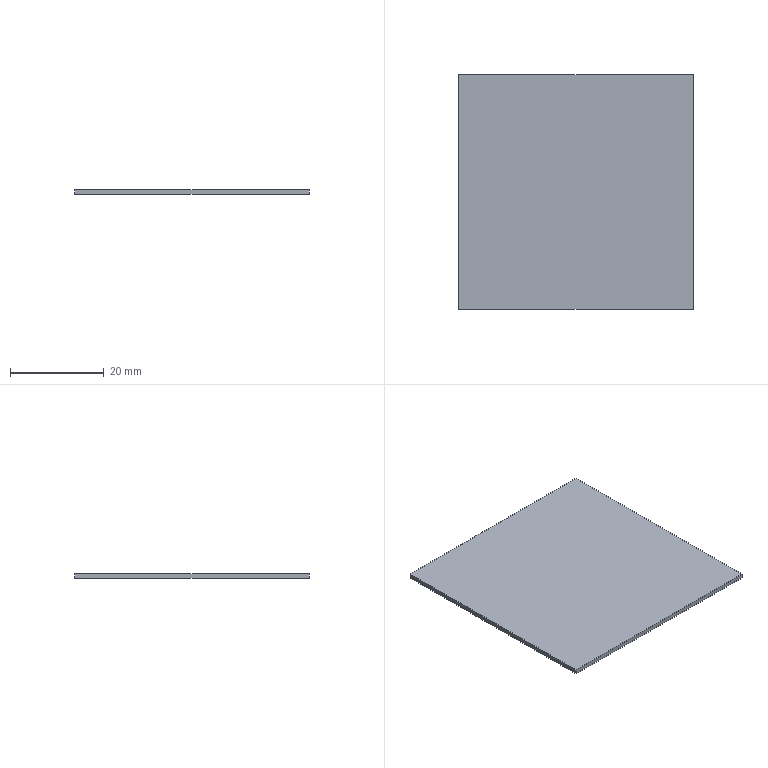Part | SolidWorks | features Extrusion 1 | 1 solid | 6 faces | box 50 x 50 x 1 mm | volume 2500 mm3 | plane 6
STEP:
#1=CARTESIAN_POINT('',(25.,-25.,0.));
#2=VERTEX_POINT('',#1);
#3=CARTESIAN_POINT('',(25.,25.,0.));
#4=VERTEX_POINT('',#3);
#5=CARTESIAN_POINT('',(25.,-25.,0.));
#6=DIRECTION('',(0.,1.,0.));
#7=VECTOR('',#6,1000.);
#8=LINE('',#5,#7);
#9=EDGE_CURVE('',#2,#4,#8,.T.);
#10=ORIENTED_EDGE('',*,*,#9,.T.);
#11=CARTESIAN_POINT('',(25.,25.,1.));
#12=VERTEX_POINT('',#11);
#13=CARTESIAN_POINT('',(25.,25.,1.));
#14=DIRECTION('',(0.,0.,-1.));
#15=VECTOR('',#14,1000.);
#16=LINE('',#13,#15);
#17=EDGE_CURVE('',#12,#4,#16,.T.);
#18=ORIENTED_EDGE('',*,*,#17,.F.);
#19=CARTESIAN_POINT('',(25.,-25.,1.));
#20=VERTEX_POINT('',#19);
#21=CARTESIAN_POINT('',(25.,-25.,1.));
#22=DIRECTION('',(0.,1.,0.));
#23=VECTOR('',#22,1000.);
#24=LINE('',#21,#23);
#25=EDGE_CURVE('',#20,#12,#24,.T.);
#26=ORIENTED_EDGE('',*,*,#25,.F.);
#27=CARTESIAN_POINT('',(25.,-25.,1.));
#28=DIRECTION('',(0.,0.,-1.));
#29=VECTOR('',#28,1000.);
#30=LINE('',#27,#29);
#31=EDGE_CURVE('',#20,#2,#30,.T.);
#32=ORIENTED_EDGE('',*,*,#31,.T.);
#33=EDGE_LOOP('',(#10,#18,#26,#32));
#34=FACE_OUTER_BOUND('',#33,.T.);
#35=CARTESIAN_POINT('',(25.,-25.,1.));
#36=DIRECTION('',(-1.,0.,0.));
#37=DIRECTION('',(0.,0.,1.));
#38=AXIS2_PLACEMENT_3D('',#35,#36,#37);
#39=PLANE('',#38);
#40=ADVANCED_FACE('',(#34),#39,.F.);
#41=CARTESIAN_POINT('',(-25.,25.,0.));
#42=VERTEX_POINT('',#41);
#43=CARTESIAN_POINT('',(-25.,25.,0.));
#44=DIRECTION('',(-1.,0.,0.));
#45=VECTOR('',#44,1000.);
#46=LINE('',#43,#45);
#47=EDGE_CURVE('',#4,#42,#46,.T.);
#48=ORIENTED_EDGE('',*,*,#47,.T.);
#49=CARTESIAN_POINT('',(-25.,25.,1.));
#50=VERTEX_POINT('',#49);
#51=CARTESIAN_POINT('',(-25.,25.,1.));
#52=DIRECTION('',(0.,0.,-1.));
#53=VECTOR('',#52,1000.);
#54=LINE('',#51,#53);
#55=EDGE_CURVE('',#50,#42,#54,.T.);
#56=ORIENTED_EDGE('',*,*,#55,.F.);
#57=CARTESIAN_POINT('',(-25.,25.,1.));
#58=DIRECTION('',(-1.,0.,0.));
#59=VECTOR('',#58,1000.);
#60=LINE('',#57,#59);
#61=EDGE_CURVE('',#12,#50,#60,.T.);
#62=ORIENTED_EDGE('',*,*,#61,.F.);
#63=ORIENTED_EDGE('',*,*,#17,.T.);
#64=EDGE_LOOP('',(#48,#56,#62,#63));
#65=FACE_OUTER_BOUND('',#64,.T.);
#66=CARTESIAN_POINT('',(-25.,25.,1.));
#67=DIRECTION('',(0.,-1.,0.));
#68=DIRECTION('',(0.,0.,-1.));
#69=AXIS2_PLACEMENT_3D('',#66,#67,#68);
#70=PLANE('',#69);
#71=ADVANCED_FACE('',(#65),#70,.F.);
#72=CARTESIAN_POINT('',(-25.,-25.,0.));
#73=VERTEX_POINT('',#72);
#74=CARTESIAN_POINT('',(-25.,-25.,0.));
#75=DIRECTION('',(0.,-1.,0.));
#76=VECTOR('',#75,1000.);
#77=LINE('',#74,#76);
#78=EDGE_CURVE('',#42,#73,#77,.T.);
#79=ORIENTED_EDGE('',*,*,#78,.T.);
#80=CARTESIAN_POINT('',(-25.,-25.,1.));
#81=VERTEX_POINT('',#80);
#82=CARTESIAN_POINT('',(-25.,-25.,1.));
#83=DIRECTION('',(0.,0.,-1.));
#84=VECTOR('',#83,1000.);
#85=LINE('',#82,#84);
#86=EDGE_CURVE('',#81,#73,#85,.T.);
#87=ORIENTED_EDGE('',*,*,#86,.F.);
#88=CARTESIAN_POINT('',(-25.,-25.,1.));
#89=DIRECTION('',(0.,-1.,0.));
#90=VECTOR('',#89,1000.);
#91=LINE('',#88,#90);
#92=EDGE_CURVE('',#50,#81,#91,.T.);
#93=ORIENTED_EDGE('',*,*,#92,.F.);
#94=ORIENTED_EDGE('',*,*,#55,.T.);
#95=EDGE_LOOP('',(#79,#87,#93,#94));
#96=FACE_OUTER_BOUND('',#95,.T.);
#97=CARTESIAN_POINT('',(-25.,-25.,1.));
#98=DIRECTION('',(1.,0.,0.));
#99=DIRECTION('',(0.,0.,-1.));
#100=AXIS2_PLACEMENT_3D('',#97,#98,#99);
#101=PLANE('',#100);
#102=ADVANCED_FACE('',(#96),#101,.F.);
#103=CARTESIAN_POINT('',(-25.,-25.,0.));
#104=DIRECTION('',(1.,0.,0.));
#105=VECTOR('',#104,1000.);
#106=LINE('',#103,#105);
#107=EDGE_CURVE('',#73,#2,#106,.T.);
#108=ORIENTED_EDGE('',*,*,#107,.T.);
#109=ORIENTED_EDGE('',*,*,#31,.F.);
#110=CARTESIAN_POINT('',(-25.,-25.,1.));
#111=DIRECTION('',(1.,0.,0.));
#112=VECTOR('',#111,1000.);
#113=LINE('',#110,#112);
#114=EDGE_CURVE('',#81,#20,#113,.T.);
#115=ORIENTED_EDGE('',*,*,#114,.F.);
#116=ORIENTED_EDGE('',*,*,#86,.T.);
#117=EDGE_LOOP('',(#108,#109,#115,#116));
#118=FACE_OUTER_BOUND('',#117,.T.);
#119=CARTESIAN_POINT('',(-25.,-25.,1.));
#120=DIRECTION('',(0.,1.,0.));
#121=DIRECTION('',(0.,0.,1.));
#122=AXIS2_PLACEMENT_3D('',#119,#120,#121);
#123=PLANE('',#122);
#124=ADVANCED_FACE('',(#118),#123,.F.);
#125=ORIENTED_EDGE('',*,*,#25,.T.);
#126=ORIENTED_EDGE('',*,*,#61,.T.);
#127=ORIENTED_EDGE('',*,*,#92,.T.);
#128=ORIENTED_EDGE('',*,*,#114,.T.);
#129=EDGE_LOOP('',(#125,#126,#127,#128));
#130=FACE_OUTER_BOUND('',#129,.T.);
#131=CARTESIAN_POINT('',(0.,0.,1.));
#132=DIRECTION('',(0.,0.,-1.));
#133=DIRECTION('',(-1.,0.,0.));
#134=AXIS2_PLACEMENT_3D('',#131,#132,#133);
#135=PLANE('',#134);
#136=ADVANCED_FACE('',(#130),#135,.F.);
#137=ORIENTED_EDGE('',*,*,#9,.F.);
#138=ORIENTED_EDGE('',*,*,#107,.F.);
#139=ORIENTED_EDGE('',*,*,#78,.F.);
#140=ORIENTED_EDGE('',*,*,#47,.F.);
#141=EDGE_LOOP('',(#137,#138,#139,#140));
#142=FACE_OUTER_BOUND('',#141,.T.);
#143=CARTESIAN_POINT('',(0.,0.,0.));
#144=DIRECTION('',(0.,0.,-1.));
#145=DIRECTION('',(-1.,0.,0.));
#146=AXIS2_PLACEMENT_3D('',#143,#144,#145);
#147=PLANE('',#146);
#148=ADVANCED_FACE('',(#142),#147,.T.);
#149=CLOSED_SHELL('',(#40,#71,#102,#124,#136,#148));
#150=MANIFOLD_SOLID_BREP('',#149);
#151=CARTESIAN_POINT('',(0.,0.,0.));
#152=DIRECTION('',(0.,0.,1.));
#153=DIRECTION('',(1.,0.,0.));
#154=AXIS2_PLACEMENT_3D('',#151,#152,#153);
#155=(LENGTH_UNIT()NAMED_UNIT(*)SI_UNIT(.MILLI.,.METRE.));
#156=UNCERTAINTY_MEASURE_WITH_UNIT(LENGTH_MEASURE(0.00001),#155,'','');
#157=(NAMED_UNIT(*)PLANE_ANGLE_UNIT()SI_UNIT($,.RADIAN.));
#158=(NAMED_UNIT(*)SI_UNIT($,.STERADIAN.)SOLID_ANGLE_UNIT());
#159=(GEOMETRIC_REPRESENTATION_CONTEXT(3)GLOBAL_UNCERTAINTY_ASSIGNED_CONTEXT((#156))GLOBAL_UNIT_ASSIGNED_CONTEXT((#155,#157,#158))REPRESENTATION_CONTEXT('',''));
#160=ADVANCED_BREP_SHAPE_REPRESENTATION('',(#150,#154),#159);